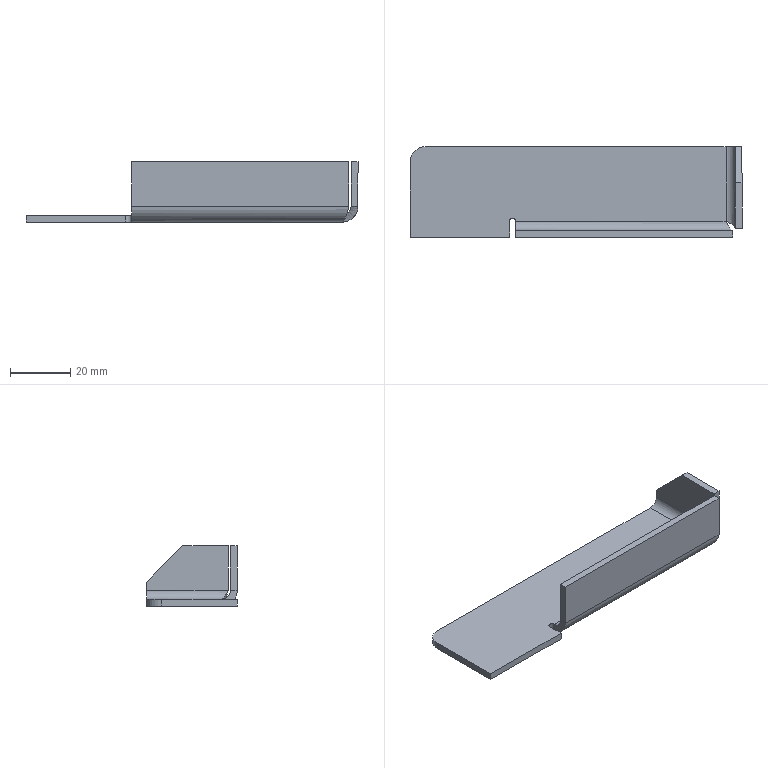Part | SolidWorks | features Chamfer 1, EdgeFlange 1, FlatPattern 1, SMBaseFlange 1, SheetMetal 1 | 1 solid | 27 faces | box 110 x 30 x 20 mm | volume 10965 mm3 | plane 19 | cylinder 6 | spline 2 | commonest cylinder face diameters 6 x2 10.6 x2 2 x1 10 x1
STEP:
#1=CARTESIAN_POINT('',(104.7,30.,-2.3));
#2=VERTEX_POINT('',#1);
#3=CARTESIAN_POINT('',(104.7,5.3,-2.3));
#4=VERTEX_POINT('',#3);
#5=CARTESIAN_POINT('',(104.7,30.,-2.3));
#6=DIRECTION('',(0.,-1.,0.));
#7=VECTOR('',#6,1000.);
#8=LINE('',#5,#7);
#9=EDGE_CURVE('',#2,#4,#8,.T.);
#10=ORIENTED_EDGE('',*,*,#9,.T.);
#11=CARTESIAN_POINT('',(35.,5.3,-2.3));
#12=VERTEX_POINT('',#11);
#13=CARTESIAN_POINT('',(106.993,5.3,-2.3));
#14=DIRECTION('',(-1.,0.,0.));
#15=VECTOR('',#14,1000.);
#16=LINE('',#13,#15);
#17=EDGE_CURVE('',#4,#12,#16,.T.);
#18=ORIENTED_EDGE('',*,*,#17,.T.);
#19=CARTESIAN_POINT('',(33.,5.3,-2.3));
#20=VERTEX_POINT('',#19);
#21=CARTESIAN_POINT('',(34.,5.3,-2.3));
#22=DIRECTION('',(0.,0.,-1.));
#23=DIRECTION('',(1.,0.,0.));
#24=AXIS2_PLACEMENT_3D('',#21,#22,#23);
#25=CIRCLE('',#24,1.);
#26=EDGE_CURVE('',#20,#12,#25,.T.);
#27=ORIENTED_EDGE('',*,*,#26,.F.);
#28=CARTESIAN_POINT('',(33.,0.,-2.3));
#29=VERTEX_POINT('',#28);
#30=CARTESIAN_POINT('',(33.,0.,-2.3));
#31=DIRECTION('',(0.,1.,0.));
#32=VECTOR('',#31,1000.);
#33=LINE('',#30,#32);
#34=EDGE_CURVE('',#29,#20,#33,.T.);
#35=ORIENTED_EDGE('',*,*,#34,.F.);
#36=CARTESIAN_POINT('',(0.,0.,-2.3));
#37=VERTEX_POINT('',#36);
#38=CARTESIAN_POINT('',(0.,0.,-2.3));
#39=DIRECTION('',(1.,0.,0.));
#40=VECTOR('',#39,1000.);
#41=LINE('',#38,#40);
#42=EDGE_CURVE('',#37,#29,#41,.T.);
#43=ORIENTED_EDGE('',*,*,#42,.F.);
#44=CARTESIAN_POINT('',(0.,25.,-2.3));
#45=VERTEX_POINT('',#44);
#46=CARTESIAN_POINT('',(0.,25.,-2.3));
#47=DIRECTION('',(0.,-1.,0.));
#48=VECTOR('',#47,1000.);
#49=LINE('',#46,#48);
#50=EDGE_CURVE('',#45,#37,#49,.T.);
#51=ORIENTED_EDGE('',*,*,#50,.F.);
#52=CARTESIAN_POINT('',(5.,30.,-2.3));
#53=VERTEX_POINT('',#52);
#54=CARTESIAN_POINT('',(5.,25.,-2.3));
#55=DIRECTION('',(0.,0.,1.));
#56=DIRECTION('',(1.,0.,0.));
#57=AXIS2_PLACEMENT_3D('',#54,#55,#56);
#58=CIRCLE('',#57,5.);
#59=EDGE_CURVE('',#53,#45,#58,.T.);
#60=ORIENTED_EDGE('',*,*,#59,.F.);
#61=CARTESIAN_POINT('',(110.,30.,-2.3));
#62=DIRECTION('',(-1.,0.,0.));
#63=VECTOR('',#62,1000.);
#64=LINE('',#61,#63);
#65=EDGE_CURVE('',#2,#53,#64,.T.);
#66=ORIENTED_EDGE('',*,*,#65,.F.);
#67=EDGE_LOOP('',(#10,#18,#27,#35,#43,#51,#60,#66));
#68=FACE_OUTER_BOUND('',#67,.T.);
#69=CARTESIAN_POINT('',(34.,5.3,-2.3));
#70=DIRECTION('',(0.,0.,1.));
#71=DIRECTION('',(1.,0.,0.));
#72=AXIS2_PLACEMENT_3D('',#69,#70,#71);
#73=PLANE('',#72);
#74=ADVANCED_FACE('',(#68),#73,.F.);
#75=CARTESIAN_POINT('',(104.7,5.3,0.));
#76=VERTEX_POINT('',#75);
#77=CARTESIAN_POINT('',(35.,5.3,0.));
#78=VERTEX_POINT('',#77);
#79=CARTESIAN_POINT('',(106.993,5.3,0.));
#80=DIRECTION('',(-1.,0.,0.));
#81=VECTOR('',#80,1000.);
#82=LINE('',#79,#81);
#83=EDGE_CURVE('',#76,#78,#82,.T.);
#84=ORIENTED_EDGE('',*,*,#83,.F.);
#85=CARTESIAN_POINT('',(104.7,30.,0.));
#86=VERTEX_POINT('',#85);
#87=CARTESIAN_POINT('',(104.7,30.,0.));
#88=DIRECTION('',(0.,-1.,0.));
#89=VECTOR('',#88,1000.);
#90=LINE('',#87,#89);
#91=EDGE_CURVE('',#86,#76,#90,.T.);
#92=ORIENTED_EDGE('',*,*,#91,.F.);
#93=CARTESIAN_POINT('',(5.,30.,0.));
#94=VERTEX_POINT('',#93);
#95=CARTESIAN_POINT('',(110.,30.,0.));
#96=DIRECTION('',(-1.,0.,0.));
#97=VECTOR('',#96,1000.);
#98=LINE('',#95,#97);
#99=EDGE_CURVE('',#86,#94,#98,.T.);
#100=ORIENTED_EDGE('',*,*,#99,.T.);
#101=CARTESIAN_POINT('',(0.,25.,0.));
#102=VERTEX_POINT('',#101);
#103=CARTESIAN_POINT('',(5.,25.,0.));
#104=DIRECTION('',(0.,0.,1.));
#105=DIRECTION('',(1.,0.,0.));
#106=AXIS2_PLACEMENT_3D('',#103,#104,#105);
#107=CIRCLE('',#106,5.);
#108=EDGE_CURVE('',#94,#102,#107,.T.);
#109=ORIENTED_EDGE('',*,*,#108,.T.);
#110=CARTESIAN_POINT('',(0.,0.,0.));
#111=VERTEX_POINT('',#110);
#112=CARTESIAN_POINT('',(0.,25.,0.));
#113=DIRECTION('',(0.,-1.,0.));
#114=VECTOR('',#113,1000.);
#115=LINE('',#112,#114);
#116=EDGE_CURVE('',#102,#111,#115,.T.);
#117=ORIENTED_EDGE('',*,*,#116,.T.);
#118=CARTESIAN_POINT('',(33.,0.,0.));
#119=VERTEX_POINT('',#118);
#120=CARTESIAN_POINT('',(0.,0.,0.));
#121=DIRECTION('',(1.,0.,0.));
#122=VECTOR('',#121,1000.);
#123=LINE('',#120,#122);
#124=EDGE_CURVE('',#111,#119,#123,.T.);
#125=ORIENTED_EDGE('',*,*,#124,.T.);
#126=CARTESIAN_POINT('',(33.,5.3,0.));
#127=VERTEX_POINT('',#126);
#128=CARTESIAN_POINT('',(33.,0.,0.));
#129=DIRECTION('',(0.,1.,0.));
#130=VECTOR('',#129,1000.);
#131=LINE('',#128,#130);
#132=EDGE_CURVE('',#119,#127,#131,.T.);
#133=ORIENTED_EDGE('',*,*,#132,.T.);
#134=CARTESIAN_POINT('',(34.,5.3,0.));
#135=DIRECTION('',(0.,0.,-1.));
#136=DIRECTION('',(1.,0.,0.));
#137=AXIS2_PLACEMENT_3D('',#134,#135,#136);
#138=CIRCLE('',#137,1.);
#139=EDGE_CURVE('',#127,#78,#138,.T.);
#140=ORIENTED_EDGE('',*,*,#139,.T.);
#141=EDGE_LOOP('',(#84,#92,#100,#109,#117,#125,#133,#140));
#142=FACE_OUTER_BOUND('',#141,.T.);
#143=CARTESIAN_POINT('',(34.,5.3,0.));
#144=DIRECTION('',(0.,0.,1.));
#145=DIRECTION('',(1.,0.,0.));
#146=AXIS2_PLACEMENT_3D('',#143,#144,#145);
#147=PLANE('',#146);
#148=ADVANCED_FACE('',(#142),#147,.T.);
#149=ORIENTED_EDGE('',*,*,#99,.F.);
#150=CARTESIAN_POINT('',(104.7,30.,0.));
#151=DIRECTION('',(0.,0.,-1.));
#152=VECTOR('',#151,1000.);
#153=LINE('',#150,#152);
#154=EDGE_CURVE('',#86,#2,#153,.T.);
#155=ORIENTED_EDGE('',*,*,#154,.T.);
#156=ORIENTED_EDGE('',*,*,#65,.T.);
#157=CARTESIAN_POINT('',(5.,30.,-2.3));
#158=DIRECTION('',(0.,0.,1.));
#159=VECTOR('',#158,1000.);
#160=LINE('',#157,#159);
#161=EDGE_CURVE('',#53,#94,#160,.T.);
#162=ORIENTED_EDGE('',*,*,#161,.T.);
#163=EDGE_LOOP('',(#149,#155,#156,#162));
#164=FACE_OUTER_BOUND('',#163,.T.);
#165=CARTESIAN_POINT('',(110.,30.,-2.3));
#166=DIRECTION('',(0.,1.,0.));
#167=DIRECTION('',(-1.,0.,0.));
#168=AXIS2_PLACEMENT_3D('',#165,#166,#167);
#169=PLANE('',#168);
#170=ADVANCED_FACE('',(#164),#169,.T.);
#171=ORIENTED_EDGE('',*,*,#116,.F.);
#172=CARTESIAN_POINT('',(0.,25.,-2.3));
#173=DIRECTION('',(0.,0.,1.));
#174=VECTOR('',#173,1000.);
#175=LINE('',#172,#174);
#176=EDGE_CURVE('',#45,#102,#175,.T.);
#177=ORIENTED_EDGE('',*,*,#176,.F.);
#178=ORIENTED_EDGE('',*,*,#50,.T.);
#179=CARTESIAN_POINT('',(0.,0.,-2.3));
#180=DIRECTION('',(0.,0.,1.));
#181=VECTOR('',#180,1000.);
#182=LINE('',#179,#181);
#183=EDGE_CURVE('',#37,#111,#182,.T.);
#184=ORIENTED_EDGE('',*,*,#183,.T.);
#185=EDGE_LOOP('',(#171,#177,#178,#184));
#186=FACE_OUTER_BOUND('',#185,.T.);
#187=CARTESIAN_POINT('',(0.,25.,-2.3));
#188=DIRECTION('',(-1.,0.,0.));
#189=DIRECTION('',(0.,0.,1.));
#190=AXIS2_PLACEMENT_3D('',#187,#188,#189);
#191=PLANE('',#190);
#192=ADVANCED_FACE('',(#186),#191,.T.);
#193=ORIENTED_EDGE('',*,*,#108,.F.);
#194=ORIENTED_EDGE('',*,*,#161,.F.);
#195=ORIENTED_EDGE('',*,*,#59,.T.);
#196=ORIENTED_EDGE('',*,*,#176,.T.);
#197=EDGE_LOOP('',(#193,#194,#195,#196));
#198=FACE_OUTER_BOUND('',#197,.T.);
#199=CARTESIAN_POINT('',(5.,25.,-2.3));
#200=DIRECTION('',(0.,0.,1.));
#201=DIRECTION('',(1.,0.,0.));
#202=AXIS2_PLACEMENT_3D('',#199,#200,#201);
#203=CYLINDRICAL_SURFACE('',#202,5.);
#204=ADVANCED_FACE('',(#198),#203,.T.);
#205=ORIENTED_EDGE('',*,*,#139,.F.);
#206=CARTESIAN_POINT('',(33.,5.3,-2.3));
#207=DIRECTION('',(0.,0.,1.));
#208=VECTOR('',#207,1000.);
#209=LINE('',#206,#208);
#210=EDGE_CURVE('',#20,#127,#209,.T.);
#211=ORIENTED_EDGE('',*,*,#210,.F.);
#212=ORIENTED_EDGE('',*,*,#26,.T.);
#213=CARTESIAN_POINT('',(35.,5.3,-2.3));
#214=DIRECTION('',(0.,0.,1.));
#215=VECTOR('',#214,1000.);
#216=LINE('',#213,#215);
#217=EDGE_CURVE('',#12,#78,#216,.T.);
#218=ORIENTED_EDGE('',*,*,#217,.T.);
#219=EDGE_LOOP('',(#205,#211,#212,#218));
#220=FACE_OUTER_BOUND('',#219,.T.);
#221=CARTESIAN_POINT('',(34.,5.3,-2.3));
#222=DIRECTION('',(0.,0.,1.));
#223=DIRECTION('',(1.,0.,0.));
#224=AXIS2_PLACEMENT_3D('',#221,#222,#223);
#225=CYLINDRICAL_SURFACE('',#224,1.);
#226=ADVANCED_FACE('',(#220),#225,.F.);
#227=ORIENTED_EDGE('',*,*,#132,.F.);
#228=CARTESIAN_POINT('',(33.,0.,-2.3));
#229=DIRECTION('',(0.,0.,1.));
#230=VECTOR('',#229,1000.);
#231=LINE('',#228,#230);
#232=EDGE_CURVE('',#29,#119,#231,.T.);
#233=ORIENTED_EDGE('',*,*,#232,.F.);
#234=ORIENTED_EDGE('',*,*,#34,.T.);
#235=ORIENTED_EDGE('',*,*,#210,.T.);
#236=EDGE_LOOP('',(#227,#233,#234,#235));
#237=FACE_OUTER_BOUND('',#236,.T.);
#238=CARTESIAN_POINT('',(33.,0.,-2.3));
#239=DIRECTION('',(1.,0.,0.));
#240=DIRECTION('',(0.,1.,0.));
#241=AXIS2_PLACEMENT_3D('',#238,#239,#240);
#242=PLANE('',#241);
#243=ADVANCED_FACE('',(#237),#242,.T.);
#244=ORIENTED_EDGE('',*,*,#124,.F.);
#245=ORIENTED_EDGE('',*,*,#183,.F.);
#246=ORIENTED_EDGE('',*,*,#42,.T.);
#247=ORIENTED_EDGE('',*,*,#232,.T.);
#248=EDGE_LOOP('',(#244,#245,#246,#247));
#249=FACE_OUTER_BOUND('',#248,.T.);
#250=CARTESIAN_POINT('',(0.,0.,-2.3));
#251=DIRECTION('',(0.,-1.,0.));
#252=DIRECTION('',(0.,0.,-1.));
#253=AXIS2_PLACEMENT_3D('',#250,#251,#252);
#254=PLANE('',#253);
#255=ADVANCED_FACE('',(#249),#254,.T.);
#256=CARTESIAN_POINT('',(35.,2.3,3.));
#257=VERTEX_POINT('',#256);
#258=CARTESIAN_POINT('',(35.,0.,3.));
#259=VERTEX_POINT('',#258);
#260=CARTESIAN_POINT('',(35.,0.,3.));
#261=DIRECTION('',(0.,-1.,0.));
#262=VECTOR('',#261,1000.);
#263=LINE('',#260,#262);
#264=EDGE_CURVE('',#257,#259,#263,.T.);
#265=ORIENTED_EDGE('',*,*,#264,.F.);
#266=CARTESIAN_POINT('',(35.,5.3,3.));
#267=DIRECTION('',(-1.,0.,0.));
#268=DIRECTION('',(0.,0.,-1.));
#269=AXIS2_PLACEMENT_3D('',#266,#267,#268);
#270=CIRCLE('',#269,3.);
#271=EDGE_CURVE('',#78,#257,#270,.T.);
#272=ORIENTED_EDGE('',*,*,#271,.F.);
#273=ORIENTED_EDGE('',*,*,#217,.F.);
#274=CARTESIAN_POINT('',(35.,5.3,3.));
#275=DIRECTION('',(-1.,0.,0.));
#276=DIRECTION('',(0.,0.,-1.));
#277=AXIS2_PLACEMENT_3D('',#274,#275,#276);
#278=CIRCLE('',#277,5.3);
#279=EDGE_CURVE('',#12,#259,#278,.T.);
#280=ORIENTED_EDGE('',*,*,#279,.T.);
#281=EDGE_LOOP('',(#265,#272,#273,#280));
#282=FACE_OUTER_BOUND('',#281,.T.);
#283=CARTESIAN_POINT('',(35.,5.3,3.));
#284=DIRECTION('',(-1.,0.,0.));
#285=DIRECTION('',(0.,0.,1.));
#286=AXIS2_PLACEMENT_3D('',#283,#284,#285);
#287=PLANE('',#286);
#288=ADVANCED_FACE('',(#282),#287,.T.);
#289=CARTESIAN_POINT('',(106.993,2.3,3.));
#290=VERTEX_POINT('',#289);
#291=CARTESIAN_POINT('',(106.993,2.3,3.));
#292=CARTESIAN_POINT('',(106.897,2.3,2.802));
#293=CARTESIAN_POINT('',(106.801,2.319,2.607));
#294=CARTESIAN_POINT('',(106.611,2.396,2.223));
#295=CARTESIAN_POINT('',(106.515,2.453,2.033));
#296=CARTESIAN_POINT('',(106.323,2.604,1.669));
#297=CARTESIAN_POINT('',(106.229,2.697,1.497));
#298=CARTESIAN_POINT('',(106.038,2.914,1.171));
#299=CARTESIAN_POINT('',(105.942,3.04,1.018));
#300=CARTESIAN_POINT('',(105.751,3.318,0.7394));
#301=CARTESIAN_POINT('',(105.656,3.469,0.6154));
#302=CARTESIAN_POINT('',(105.466,3.794,0.3979));
#303=CARTESIAN_POINT('',(105.369,3.97,0.3037));
#304=CARTESIAN_POINT('',(105.178,4.333,0.1534));
#305=CARTESIAN_POINT('',(105.083,4.52,0.09658));
#306=CARTESIAN_POINT('',(104.893,4.904,0.01983));
#307=CARTESIAN_POINT('',(104.796,5.102,0.));
#308=CARTESIAN_POINT('',(104.7,5.3,0.));
#309=B_SPLINE_CURVE_WITH_KNOTS('',3,(#291,#292,#293,#294,#295,#296,#297,#298,#299,#300,#301,#302,#303,#304,#305,#306,#307,#308),.UNSPECIFIED.,.F.,.F.,(4,2,2,2,2,2,2,2,4),(0.,0.0006524,0.001305,0.001957,0.00261,0.003262,0.003914,0.004567,0.005219),.UNSPECIFIED.);
#310=EDGE_CURVE('',#290,#76,#309,.T.);
#311=ORIENTED_EDGE('',*,*,#310,.F.);
#312=CARTESIAN_POINT('',(106.993,0.,3.));
#313=VERTEX_POINT('',#312);
#314=CARTESIAN_POINT('',(106.993,2.3,3.));
#315=DIRECTION('',(0.,1.,0.));
#316=VECTOR('',#315,1000.);
#317=LINE('',#314,#316);
#318=EDGE_CURVE('',#313,#290,#317,.T.);
#319=ORIENTED_EDGE('',*,*,#318,.F.);
#320=CARTESIAN_POINT('',(106.993,0.,3.));
#321=CARTESIAN_POINT('',(106.897,0.,2.65));
#322=CARTESIAN_POINT('',(106.802,0.03435,2.306));
#323=CARTESIAN_POINT('',(106.659,0.1352,1.798));
#324=CARTESIAN_POINT('',(106.612,0.1771,1.63));
#325=CARTESIAN_POINT('',(106.516,0.2777,1.298));
#326=CARTESIAN_POINT('',(106.468,0.3368,1.133));
#327=CARTESIAN_POINT('',(106.324,0.5364,0.6506));
#328=CARTESIAN_POINT('',(106.229,0.6993,0.3462));
#329=CARTESIAN_POINT('',(106.039,1.083,-0.2288));
#330=CARTESIAN_POINT('',(105.942,1.306,-0.5016));
#331=CARTESIAN_POINT('',(105.752,1.796,-0.9914));
#332=CARTESIAN_POINT('',(105.657,2.063,-1.211));
#333=CARTESIAN_POINT('',(105.466,2.639,-1.597));
#334=CARTESIAN_POINT('',(105.369,2.949,-1.763));
#335=CARTESIAN_POINT('',(105.179,3.587,-2.027));
#336=CARTESIAN_POINT('',(105.084,3.918,-2.128));
#337=CARTESIAN_POINT('',(104.893,4.601,-2.265));
#338=CARTESIAN_POINT('',(104.796,4.95,-2.3));
#339=CARTESIAN_POINT('',(104.7,5.3,-2.3));
#340=B_SPLINE_CURVE_WITH_KNOTS('',3,(#320,#321,#322,#323,#324,#325,#326,#327,#328,#329,#330,#331,#332,#333,#334,#335,#336,#337,#338,#339),.UNSPECIFIED.,.F.,.F.,(4,2,2,2,2,2,2,2,2,4),(0.,0.001073,0.00161,0.002147,0.00322,0.004294,0.005367,0.006441,0.007514,0.008588),.UNSPECIFIED.);
#341=EDGE_CURVE('',#313,#4,#340,.T.);
#342=ORIENTED_EDGE('',*,*,#341,.T.);
#343=CARTESIAN_POINT('',(104.7,5.3,0.));
#344=DIRECTION('',(0.,0.,-1.));
#345=VECTOR('',#344,1000.);
#346=LINE('',#343,#345);
#347=EDGE_CURVE('',#76,#4,#346,.T.);
#348=ORIENTED_EDGE('',*,*,#347,.F.);
#349=EDGE_LOOP('',(#311,#319,#342,#348));
#350=FACE_OUTER_BOUND('',#349,.T.);
#351=CARTESIAN_POINT('',(106.993,-0.023,3.));
#352=CARTESIAN_POINT('',(106.802,-0.023,2.303));
#353=CARTESIAN_POINT('',(106.611,0.1155,1.607));
#354=CARTESIAN_POINT('',(106.229,0.6488,0.3192));
#355=CARTESIAN_POINT('',(106.038,1.043,-0.2712));
#356=CARTESIAN_POINT('',(105.655,2.029,-1.257));
#357=CARTESIAN_POINT('',(105.464,2.619,-1.651));
#358=CARTESIAN_POINT('',(105.082,3.907,-2.184));
#359=CARTESIAN_POINT('',(104.891,4.603,-2.323));
#360=CARTESIAN_POINT('',(104.7,5.3,-2.323));
#361=CARTESIAN_POINT('',(106.993,0.,3.));
#362=CARTESIAN_POINT('',(106.802,0.,2.306));
#363=CARTESIAN_POINT('',(106.611,0.1379,1.613));
#364=CARTESIAN_POINT('',(106.229,0.6689,0.3308));
#365=CARTESIAN_POINT('',(106.038,1.062,-0.2571));
#366=CARTESIAN_POINT('',(105.655,2.043,-1.238));
#367=CARTESIAN_POINT('',(105.464,2.631,-1.631));
#368=CARTESIAN_POINT('',(105.082,3.913,-2.162));
#369=CARTESIAN_POINT('',(104.891,4.606,-2.3));
#370=CARTESIAN_POINT('',(104.7,5.3,-2.3));
#371=CARTESIAN_POINT('',(106.993,2.3,3.));
#372=CARTESIAN_POINT('',(106.802,2.3,2.607));
#373=CARTESIAN_POINT('',(106.611,2.378,2.215));
#374=CARTESIAN_POINT('',(106.229,2.679,1.489));
#375=CARTESIAN_POINT('',(106.038,2.901,1.156));
#376=CARTESIAN_POINT('',(105.655,3.456,0.601));
#377=CARTESIAN_POINT('',(105.464,3.789,0.3786));
#378=CARTESIAN_POINT('',(105.082,4.515,0.07808));
#379=CARTESIAN_POINT('',(104.891,4.907,0.));
#380=CARTESIAN_POINT('',(104.7,5.3,0.));
#381=CARTESIAN_POINT('',(106.993,2.323,3.));
#382=CARTESIAN_POINT('',(106.802,2.323,2.61));
#383=CARTESIAN_POINT('',(106.611,2.401,2.221));
#384=CARTESIAN_POINT('',(106.229,2.699,1.501));
#385=CARTESIAN_POINT('',(106.038,2.92,1.171));
#386=CARTESIAN_POINT('',(105.655,3.471,0.6196));
#387=CARTESIAN_POINT('',(105.464,3.801,0.3989));
#388=CARTESIAN_POINT('',(105.082,4.521,0.1007));
#389=CARTESIAN_POINT('',(104.891,4.91,0.02323));
#390=CARTESIAN_POINT('',(104.7,5.3,0.02323));
#391=B_SPLINE_SURFACE_WITH_KNOTS('',1,3,((#351,#352,#353,#354,#355,#356,#357,#358,#359,#360),(#361,#362,#363,#364,#365,#366,#367,#368,#369,#370),(#371,#372,#373,#374,#375,#376,#377,#378,#379,#380),(#381,#382,#383,#384,#385,#386,#387,#388,#389,#390)),.UNSPECIFIED.,.F.,.F.,.F.,(2,1,1,2),(4,2,2,2,4),(-0.01,0.,1.,1.01),(0.,0.25,0.5,0.75,1.),.UNSPECIFIED.);
#392=ADVANCED_FACE('',(#350),#391,.F.);
#393=ORIENTED_EDGE('',*,*,#17,.F.);
#394=ORIENTED_EDGE('',*,*,#341,.F.);
#395=CARTESIAN_POINT('',(35.,0.,3.));
#396=DIRECTION('',(-1.,0.,0.));
#397=VECTOR('',#396,1000.);
#398=LINE('',#395,#397);
#399=EDGE_CURVE('',#313,#259,#398,.T.);
#400=ORIENTED_EDGE('',*,*,#399,.T.);
#401=ORIENTED_EDGE('',*,*,#279,.F.);
#402=EDGE_LOOP('',(#393,#394,#400,#401));
#403=FACE_OUTER_BOUND('',#402,.T.);
#404=CARTESIAN_POINT('',(106.993,5.3,3.));
#405=DIRECTION('',(1.,0.,0.));
#406=DIRECTION('',(0.,-1.,0.));
#407=AXIS2_PLACEMENT_3D('',#404,#405,#406);
#408=CYLINDRICAL_SURFACE('',#407,5.3);
#409=ADVANCED_FACE('',(#403),#408,.T.);
#410=ORIENTED_EDGE('',*,*,#83,.T.);
#411=ORIENTED_EDGE('',*,*,#271,.T.);
#412=CARTESIAN_POINT('',(35.,2.3,3.));
#413=DIRECTION('',(1.,0.,0.));
#414=VECTOR('',#413,1000.);
#415=LINE('',#412,#414);
#416=EDGE_CURVE('',#257,#290,#415,.T.);
#417=ORIENTED_EDGE('',*,*,#416,.T.);
#418=ORIENTED_EDGE('',*,*,#310,.T.);
#419=EDGE_LOOP('',(#410,#411,#417,#418));
#420=FACE_OUTER_BOUND('',#419,.T.);
#421=CARTESIAN_POINT('',(106.993,5.3,3.));
#422=DIRECTION('',(1.,0.,0.));
#423=DIRECTION('',(0.,-1.,0.));
#424=AXIS2_PLACEMENT_3D('',#421,#422,#423);
#425=CYLINDRICAL_SURFACE('',#424,3.);
#426=ADVANCED_FACE('',(#420),#425,.F.);
#427=ORIENTED_EDGE('',*,*,#264,.T.);
#428=CARTESIAN_POINT('',(35.,0.,17.7));
#429=VERTEX_POINT('',#428);
#430=CARTESIAN_POINT('',(35.,0.,0.));
#431=DIRECTION('',(0.,0.,-1.));
#432=VECTOR('',#431,1000.);
#433=LINE('',#430,#432);
#434=EDGE_CURVE('',#429,#259,#433,.T.);
#435=ORIENTED_EDGE('',*,*,#434,.F.);
#436=CARTESIAN_POINT('',(35.,2.3,17.7));
#437=VERTEX_POINT('',#436);
#438=CARTESIAN_POINT('',(35.,0.,17.7));
#439=DIRECTION('',(0.,1.,0.));
#440=VECTOR('',#439,1000.);
#441=LINE('',#438,#440);
#442=EDGE_CURVE('',#429,#437,#441,.T.);
#443=ORIENTED_EDGE('',*,*,#442,.T.);
#444=CARTESIAN_POINT('',(35.,2.3,0.));
#445=DIRECTION('',(0.,0.,-1.));
#446=VECTOR('',#445,1000.);
#447=LINE('',#444,#446);
#448=EDGE_CURVE('',#437,#257,#447,.T.);
#449=ORIENTED_EDGE('',*,*,#448,.T.);
#450=EDGE_LOOP('',(#427,#435,#443,#449));
#451=FACE_OUTER_BOUND('',#450,.T.);
#452=CARTESIAN_POINT('',(35.,0.,0.));
#453=DIRECTION('',(1.,0.,0.));
#454=DIRECTION('',(0.,0.,-1.));
#455=AXIS2_PLACEMENT_3D('',#452,#453,#454);
#456=PLANE('',#455);
#457=ADVANCED_FACE('',(#451),#456,.F.);
#458=ORIENTED_EDGE('',*,*,#399,.F.);
#459=CARTESIAN_POINT('',(106.993,0.,17.7));
#460=VERTEX_POINT('',#459);
#461=CARTESIAN_POINT('',(106.993,0.,0.));
#462=DIRECTION('',(0.,0.,1.));
#463=VECTOR('',#462,1000.);
#464=LINE('',#461,#463);
#465=EDGE_CURVE('',#313,#460,#464,.T.);
#466=ORIENTED_EDGE('',*,*,#465,.T.);
#467=CARTESIAN_POINT('',(0.,0.,17.7));
#468=DIRECTION('',(-1.,0.,0.));
#469=VECTOR('',#468,1000.);
#470=LINE('',#467,#469);
#471=EDGE_CURVE('',#460,#429,#470,.T.);
#472=ORIENTED_EDGE('',*,*,#471,.T.);
#473=ORIENTED_EDGE('',*,*,#434,.T.);
#474=EDGE_LOOP('',(#458,#466,#472,#473));
#475=FACE_OUTER_BOUND('',#474,.T.);
#476=CARTESIAN_POINT('',(0.,0.,0.));
#477=DIRECTION('',(0.,1.,0.));
#478=DIRECTION('',(0.,0.,1.));
#479=AXIS2_PLACEMENT_3D('',#476,#477,#478);
#480=PLANE('',#479);
#481=ADVANCED_FACE('',(#475),#480,.F.);
#482=CARTESIAN_POINT('',(106.993,2.3,17.7));
#483=VERTEX_POINT('',#482);
#484=CARTESIAN_POINT('',(106.993,2.3,0.));
#485=DIRECTION('',(0.,0.,1.));
#486=VECTOR('',#485,1000.);
#487=LINE('',#484,#486);
#488=EDGE_CURVE('',#290,#483,#487,.T.);
#489=ORIENTED_EDGE('',*,*,#488,.F.);
#490=ORIENTED_EDGE('',*,*,#416,.F.);
#491=ORIENTED_EDGE('',*,*,#448,.F.);
#492=CARTESIAN_POINT('',(35.,2.3,17.7));
#493=DIRECTION('',(-1.,0.,0.));
#494=VECTOR('',#493,1000.);
#495=LINE('',#492,#494);
#496=EDGE_CURVE('',#483,#437,#495,.T.);
#497=ORIENTED_EDGE('',*,*,#496,.F.);
#498=EDGE_LOOP('',(#489,#490,#491,#497));
#499=FACE_OUTER_BOUND('',#498,.T.);
#500=CARTESIAN_POINT('',(0.,2.3,0.));
#501=DIRECTION('',(0.,1.,0.));
#502=DIRECTION('',(0.,0.,1.));
#503=AXIS2_PLACEMENT_3D('',#500,#501,#502);
#504=PLANE('',#503);
#505=ADVANCED_FACE('',(#499),#504,.T.);
#506=ORIENTED_EDGE('',*,*,#471,.F.);
#507=CARTESIAN_POINT('',(106.993,0.,17.7));
#508=DIRECTION('',(0.,1.,0.));
#509=VECTOR('',#508,1000.);
#510=LINE('',#507,#509);
#511=EDGE_CURVE('',#460,#483,#510,.T.);
#512=ORIENTED_EDGE('',*,*,#511,.T.);
#513=ORIENTED_EDGE('',*,*,#496,.T.);
#514=ORIENTED_EDGE('',*,*,#442,.F.);
#515=EDGE_LOOP('',(#506,#512,#513,#514));
#516=FACE_OUTER_BOUND('',#515,.T.);
#517=CARTESIAN_POINT('',(35.,0.,17.7));
#518=DIRECTION('',(0.,0.,-1.));
#519=DIRECTION('',(0.,1.,0.));
#520=AXIS2_PLACEMENT_3D('',#517,#518,#519);
#521=PLANE('',#520);
#522=ADVANCED_FACE('',(#516),#521,.F.);
#523=ORIENTED_EDGE('',*,*,#511,.F.);
#524=ORIENTED_EDGE('',*,*,#465,.F.);
#525=ORIENTED_EDGE('',*,*,#318,.T.);
#526=ORIENTED_EDGE('',*,*,#488,.T.);
#527=EDGE_LOOP('',(#523,#524,#525,#526));
#528=FACE_OUTER_BOUND('',#527,.T.);
#529=CARTESIAN_POINT('',(106.993,2.3,0.));
#530=DIRECTION('',(-1.,0.,0.));
#531=DIRECTION('',(0.,0.,1.));
#532=AXIS2_PLACEMENT_3D('',#529,#530,#531);
#533=PLANE('',#532);
#534=ADVANCED_FACE('',(#528),#533,.F.);
#535=CARTESIAN_POINT('',(110.,3.007,3.));
#536=VERTEX_POINT('',#535);
#537=CARTESIAN_POINT('',(107.7,3.007,3.));
#538=VERTEX_POINT('',#537);
#539=CARTESIAN_POINT('',(107.7,3.007,3.));
#540=DIRECTION('',(-1.,0.,0.));
#541=VECTOR('',#540,1000.);
#542=LINE('',#539,#541);
#543=EDGE_CURVE('',#536,#538,#542,.T.);
#544=ORIENTED_EDGE('',*,*,#543,.T.);
#545=CARTESIAN_POINT('',(104.7,5.3,0.));
#546=CARTESIAN_POINT('',(104.898,5.204,0.));
#547=CARTESIAN_POINT('',(105.093,5.109,0.01948));
#548=CARTESIAN_POINT('',(105.477,4.918,0.09577));
#549=CARTESIAN_POINT('',(105.667,4.822,0.1532));
#550=CARTESIAN_POINT('',(106.031,4.63,0.3042));
#551=CARTESIAN_POINT('',(106.203,4.536,0.3966));
#552=CARTESIAN_POINT('',(106.529,4.345,0.6136));
#553=CARTESIAN_POINT('',(106.682,4.249,0.7397));
#554=CARTESIAN_POINT('',(106.961,4.058,1.018));
#555=CARTESIAN_POINT('',(107.085,3.963,1.169));
#556=CARTESIAN_POINT('',(107.302,3.773,1.494));
#557=CARTESIAN_POINT('',(107.396,3.676,1.67));
#558=CARTESIAN_POINT('',(107.547,3.485,2.033));
#559=CARTESIAN_POINT('',(107.603,3.39,2.22));
#560=CARTESIAN_POINT('',(107.68,3.2,2.604));
#561=CARTESIAN_POINT('',(107.7,3.103,2.802));
#562=CARTESIAN_POINT('',(107.7,3.007,3.));
#563=B_SPLINE_CURVE_WITH_KNOTS('',3,(#545,#546,#547,#548,#549,#550,#551,#552,#553,#554,#555,#556,#557,#558,#559,#560,#561,#562),.UNSPECIFIED.,.F.,.F.,(4,2,2,2,2,2,2,2,4),(0.,0.0006524,0.001305,0.001957,0.00261,0.003262,0.003914,0.004567,0.005219),.UNSPECIFIED.);
#564=EDGE_CURVE('',#76,#538,#563,.T.);
#565=ORIENTED_EDGE('',*,*,#564,.F.);
#566=ORIENTED_EDGE('',*,*,#347,.T.);
#567=CARTESIAN_POINT('',(104.7,5.3,-2.3));
#568=CARTESIAN_POINT('',(105.05,5.204,-2.3));
#569=CARTESIAN_POINT('',(105.394,5.109,-2.266));
#570=CARTESIAN_POINT('',(105.902,4.966,-2.165));
#571=CARTESIAN_POINT('',(106.07,4.919,-2.123));
#572=CARTESIAN_POINT('',(106.402,4.823,-2.022));
#573=CARTESIAN_POINT('',(106.567,4.775,-1.963));
#574=CARTESIAN_POINT('',(107.049,4.631,-1.764));
#575=CARTESIAN_POINT('',(107.354,4.536,-1.601));
#576=CARTESIAN_POINT('',(107.929,4.346,-1.217));
#577=CARTESIAN_POINT('',(108.202,4.249,-0.9936));
#578=CARTESIAN_POINT('',(108.691,4.059,-0.504));
#579=CARTESIAN_POINT('',(108.911,3.964,-0.2375));
#580=CARTESIAN_POINT('',(109.297,3.773,0.3388));
#581=CARTESIAN_POINT('',(109.463,3.676,0.6493));
#582=CARTESIAN_POINT('',(109.727,3.486,1.287));
#583=CARTESIAN_POINT('',(109.828,3.392,1.618));
#584=CARTESIAN_POINT('',(109.965,3.2,2.301));
#585=CARTESIAN_POINT('',(110.,3.103,2.65));
#586=CARTESIAN_POINT('',(110.,3.007,3.));
#587=B_SPLINE_CURVE_WITH_KNOTS('',3,(#567,#568,#569,#570,#571,#572,#573,#574,#575,#576,#577,#578,#579,#580,#581,#582,#583,#584,#585,#586),.UNSPECIFIED.,.F.,.F.,(4,2,2,2,2,2,2,2,2,4),(0.,0.001073,0.00161,0.002147,0.00322,0.004294,0.005367,0.006441,0.007514,0.008588),.UNSPECIFIED.);
#588=EDGE_CURVE('',#4,#536,#587,.T.);
#589=ORIENTED_EDGE('',*,*,#588,.T.);
#590=EDGE_LOOP('',(#544,#565,#566,#589));
#591=FACE_OUTER_BOUND('',#590,.T.);
#592=CARTESIAN_POINT('',(104.7,5.3,-2.323));
#593=CARTESIAN_POINT('',(105.397,5.109,-2.323));
#594=CARTESIAN_POINT('',(106.093,4.918,-2.184));
#595=CARTESIAN_POINT('',(107.381,4.536,-1.651));
#596=CARTESIAN_POINT('',(107.971,4.345,-1.257));
#597=CARTESIAN_POINT('',(108.957,3.962,-0.2712));
#598=CARTESIAN_POINT('',(109.351,3.771,0.3192));
#599=CARTESIAN_POINT('',(109.884,3.389,1.607));
#600=CARTESIAN_POINT('',(110.023,3.198,2.303));
#601=CARTESIAN_POINT('',(110.023,3.007,3.));
#602=CARTESIAN_POINT('',(104.7,5.3,-2.3));
#603=CARTESIAN_POINT('',(105.394,5.109,-2.3));
#604=CARTESIAN_POINT('',(106.087,4.918,-2.162));
#605=CARTESIAN_POINT('',(107.369,4.536,-1.631));
#606=CARTESIAN_POINT('',(107.957,4.345,-1.238));
#607=CARTESIAN_POINT('',(108.938,3.962,-0.2571));
#608=CARTESIAN_POINT('',(109.331,3.771,0.3308));
#609=CARTESIAN_POINT('',(109.862,3.389,1.613));
#610=CARTESIAN_POINT('',(110.,3.198,2.306));
#611=CARTESIAN_POINT('',(110.,3.007,3.));
#612=CARTESIAN_POINT('',(104.7,5.3,0.));
#613=CARTESIAN_POINT('',(105.093,5.109,0.));
#614=CARTESIAN_POINT('',(105.485,4.918,0.07808));
#615=CARTESIAN_POINT('',(106.211,4.536,0.3786));
#616=CARTESIAN_POINT('',(106.544,4.345,0.601));
#617=CARTESIAN_POINT('',(107.099,3.962,1.156));
#618=CARTESIAN_POINT('',(107.321,3.771,1.489));
#619=CARTESIAN_POINT('',(107.622,3.389,2.215));
#620=CARTESIAN_POINT('',(107.7,3.198,2.607));
#621=CARTESIAN_POINT('',(107.7,3.007,3.));
#622=CARTESIAN_POINT('',(104.7,5.3,0.02323));
#623=CARTESIAN_POINT('',(105.09,5.109,0.02323));
#624=CARTESIAN_POINT('',(105.479,4.918,0.1007));
#625=CARTESIAN_POINT('',(106.199,4.536,0.3989));
#626=CARTESIAN_POINT('',(106.529,4.345,0.6196));
#627=CARTESIAN_POINT('',(107.08,3.962,1.171));
#628=CARTESIAN_POINT('',(107.301,3.771,1.501));
#629=CARTESIAN_POINT('',(107.599,3.389,2.221));
#630=CARTESIAN_POINT('',(107.677,3.198,2.61));
#631=CARTESIAN_POINT('',(107.677,3.007,3.));
#632=B_SPLINE_SURFACE_WITH_KNOTS('',1,3,((#592,#593,#594,#595,#596,#597,#598,#599,#600,#601),(#602,#603,#604,#605,#606,#607,#608,#609,#610,#611),(#612,#613,#614,#615,#616,#617,#618,#619,#620,#621),(#622,#623,#624,#625,#626,#627,#628,#629,#630,#631)),.UNSPECIFIED.,.F.,.F.,.F.,(2,1,1,2),(4,2,2,2,4),(-0.01,0.,1.,1.01),(0.,0.25,0.5,0.75,1.),.UNSPECIFIED.);
#633=ADVANCED_FACE('',(#591),#632,.F.);
#634=CARTESIAN_POINT('',(107.7,30.,3.));
#635=VERTEX_POINT('',#634);
#636=CARTESIAN_POINT('',(104.7,30.,3.));
#637=DIRECTION('',(0.,1.,0.));
#638=DIRECTION('',(0.,0.,1.));
#639=AXIS2_PLACEMENT_3D('',#636,#637,#638);
#640=CIRCLE('',#639,3.);
#641=EDGE_CURVE('',#635,#86,#640,.T.);
#642=ORIENTED_EDGE('',*,*,#641,.F.);
#643=CARTESIAN_POINT('',(110.,30.,3.));
#644=VERTEX_POINT('',#643);
#645=CARTESIAN_POINT('',(107.7,30.,3.));
#646=DIRECTION('',(1.,0.,0.));
#647=VECTOR('',#646,1000.);
#648=LINE('',#645,#647);
#649=EDGE_CURVE('',#635,#644,#648,.T.);
#650=ORIENTED_EDGE('',*,*,#649,.T.);
#651=CARTESIAN_POINT('',(104.7,30.,3.));
#652=DIRECTION('',(0.,1.,0.));
#653=DIRECTION('',(0.,0.,1.));
#654=AXIS2_PLACEMENT_3D('',#651,#652,#653);
#655=CIRCLE('',#654,5.3);
#656=EDGE_CURVE('',#644,#2,#655,.T.);
#657=ORIENTED_EDGE('',*,*,#656,.T.);
#658=ORIENTED_EDGE('',*,*,#154,.F.);
#659=EDGE_LOOP('',(#642,#650,#657,#658));
#660=FACE_OUTER_BOUND('',#659,.T.);
#661=CARTESIAN_POINT('',(104.7,30.,3.));
#662=DIRECTION('',(0.,-1.,0.));
#663=DIRECTION('',(0.,0.,-1.));
#664=AXIS2_PLACEMENT_3D('',#661,#662,#663);
#665=PLANE('',#664);
#666=ADVANCED_FACE('',(#660),#665,.F.);
#667=ORIENTED_EDGE('',*,*,#9,.F.);
#668=ORIENTED_EDGE('',*,*,#656,.F.);
#669=CARTESIAN_POINT('',(110.,0.,3.));
#670=DIRECTION('',(0.,-1.,0.));
#671=VECTOR('',#670,1000.);
#672=LINE('',#669,#671);
#673=EDGE_CURVE('',#644,#536,#672,.T.);
#674=ORIENTED_EDGE('',*,*,#673,.T.);
#675=ORIENTED_EDGE('',*,*,#588,.F.);
#676=EDGE_LOOP('',(#667,#668,#674,#675));
#677=FACE_OUTER_BOUND('',#676,.T.);
#678=CARTESIAN_POINT('',(104.7,30.,3.));
#679=DIRECTION('',(0.,1.,0.));
#680=DIRECTION('',(1.,0.,0.));
#681=AXIS2_PLACEMENT_3D('',#678,#679,#680);
#682=CYLINDRICAL_SURFACE('',#681,5.3);
#683=ADVANCED_FACE('',(#677),#682,.T.);
#684=ORIENTED_EDGE('',*,*,#91,.T.);
#685=ORIENTED_EDGE('',*,*,#564,.T.);
#686=CARTESIAN_POINT('',(107.7,0.,3.));
#687=DIRECTION('',(0.,1.,0.));
#688=VECTOR('',#687,1000.);
#689=LINE('',#686,#688);
#690=EDGE_CURVE('',#538,#635,#689,.T.);
#691=ORIENTED_EDGE('',*,*,#690,.T.);
#692=ORIENTED_EDGE('',*,*,#641,.T.);
#693=EDGE_LOOP('',(#684,#685,#691,#692));
#694=FACE_OUTER_BOUND('',#693,.T.);
#695=CARTESIAN_POINT('',(104.7,30.,3.));
#696=DIRECTION('',(0.,1.,0.));
#697=DIRECTION('',(1.,0.,0.));
#698=AXIS2_PLACEMENT_3D('',#695,#696,#697);
#699=CYLINDRICAL_SURFACE('',#698,3.);
#700=ADVANCED_FACE('',(#694),#699,.F.);
#701=CARTESIAN_POINT('',(110.,3.007,17.7));
#702=VERTEX_POINT('',#701);
#703=CARTESIAN_POINT('',(110.,3.007,0.));
#704=DIRECTION('',(0.,0.,1.));
#705=VECTOR('',#704,1000.);
#706=LINE('',#703,#705);
#707=EDGE_CURVE('',#536,#702,#706,.T.);
#708=ORIENTED_EDGE('',*,*,#707,.T.);
#709=CARTESIAN_POINT('',(107.7,3.007,17.7));
#710=VERTEX_POINT('',#709);
#711=CARTESIAN_POINT('',(107.7,3.007,17.7));
#712=DIRECTION('',(-1.,0.,0.));
#713=VECTOR('',#712,1000.);
#714=LINE('',#711,#713);
#715=EDGE_CURVE('',#702,#710,#714,.T.);
#716=ORIENTED_EDGE('',*,*,#715,.T.);
#717=CARTESIAN_POINT('',(107.7,3.007,0.));
#718=DIRECTION('',(0.,0.,1.));
#719=VECTOR('',#718,1000.);
#720=LINE('',#717,#719);
#721=EDGE_CURVE('',#538,#710,#720,.T.);
#722=ORIENTED_EDGE('',*,*,#721,.F.);
#723=ORIENTED_EDGE('',*,*,#543,.F.);
#724=EDGE_LOOP('',(#708,#716,#722,#723));
#725=FACE_OUTER_BOUND('',#724,.T.);
#726=CARTESIAN_POINT('',(107.7,3.007,0.));
#727=DIRECTION('',(0.,-1.,0.));
#728=DIRECTION('',(0.,0.,-1.));
#729=AXIS2_PLACEMENT_3D('',#726,#727,#728);
#730=PLANE('',#729);
#731=ADVANCED_FACE('',(#725),#730,.T.);
#732=CARTESIAN_POINT('',(110.,30.,5.7));
#733=VERTEX_POINT('',#732);
#734=CARTESIAN_POINT('',(110.,30.,0.));
#735=DIRECTION('',(0.,0.,1.));
#736=VECTOR('',#735,1000.);
#737=LINE('',#734,#736);
#738=EDGE_CURVE('',#644,#733,#737,.T.);
#739=ORIENTED_EDGE('',*,*,#738,.T.);
#740=CARTESIAN_POINT('',(110.,18.,17.7));
#741=VERTEX_POINT('',#740);
#742=CARTESIAN_POINT('',(110.,18.,17.7));
#743=DIRECTION('',(0.,-0.7071,0.7071));
#744=VECTOR('',#743,1000.);
#745=LINE('',#742,#744);
#746=EDGE_CURVE('',#733,#741,#745,.T.);
#747=ORIENTED_EDGE('',*,*,#746,.T.);
#748=CARTESIAN_POINT('',(110.,0.,17.7));
#749=DIRECTION('',(0.,-1.,0.));
#750=VECTOR('',#749,1000.);
#751=LINE('',#748,#750);
#752=EDGE_CURVE('',#741,#702,#751,.T.);
#753=ORIENTED_EDGE('',*,*,#752,.T.);
#754=ORIENTED_EDGE('',*,*,#707,.F.);
#755=ORIENTED_EDGE('',*,*,#673,.F.);
#756=EDGE_LOOP('',(#739,#747,#753,#754,#755));
#757=FACE_OUTER_BOUND('',#756,.T.);
#758=CARTESIAN_POINT('',(110.,0.,0.));
#759=DIRECTION('',(-1.,0.,0.));
#760=DIRECTION('',(0.,0.,1.));
#761=AXIS2_PLACEMENT_3D('',#758,#759,#760);
#762=PLANE('',#761);
#763=ADVANCED_FACE('',(#757),#762,.F.);
#764=CARTESIAN_POINT('',(107.7,18.,17.7));
#765=VERTEX_POINT('',#764);
#766=CARTESIAN_POINT('',(107.7,0.,17.7));
#767=DIRECTION('',(0.,-1.,0.));
#768=VECTOR('',#767,1000.);
#769=LINE('',#766,#768);
#770=EDGE_CURVE('',#765,#710,#769,.T.);
#771=ORIENTED_EDGE('',*,*,#770,.F.);
#772=CARTESIAN_POINT('',(107.7,30.,5.7));
#773=VERTEX_POINT('',#772);
#774=CARTESIAN_POINT('',(107.7,17.85,17.85));
#775=DIRECTION('',(0.,0.7071,-0.7071));
#776=VECTOR('',#775,1000.);
#777=LINE('',#774,#776);
#778=EDGE_CURVE('',#765,#773,#777,.T.);
#779=ORIENTED_EDGE('',*,*,#778,.T.);
#780=CARTESIAN_POINT('',(107.7,30.,17.7));
#781=DIRECTION('',(0.,0.,1.));
#782=VECTOR('',#781,1000.);
#783=LINE('',#780,#782);
#784=EDGE_CURVE('',#635,#773,#783,.T.);
#785=ORIENTED_EDGE('',*,*,#784,.F.);
#786=ORIENTED_EDGE('',*,*,#690,.F.);
#787=ORIENTED_EDGE('',*,*,#721,.T.);
#788=EDGE_LOOP('',(#771,#779,#785,#786,#787));
#789=FACE_OUTER_BOUND('',#788,.T.);
#790=CARTESIAN_POINT('',(107.7,0.,0.));
#791=DIRECTION('',(-1.,0.,0.));
#792=DIRECTION('',(0.,0.,1.));
#793=AXIS2_PLACEMENT_3D('',#790,#791,#792);
#794=PLANE('',#793);
#795=ADVANCED_FACE('',(#789),#794,.T.);
#796=ORIENTED_EDGE('',*,*,#752,.F.);
#797=CARTESIAN_POINT('',(110.,18.,17.7));
#798=DIRECTION('',(-1.,0.,0.));
#799=VECTOR('',#798,1000.);
#800=LINE('',#797,#799);
#801=EDGE_CURVE('',#741,#765,#800,.T.);
#802=ORIENTED_EDGE('',*,*,#801,.T.);
#803=ORIENTED_EDGE('',*,*,#770,.T.);
#804=ORIENTED_EDGE('',*,*,#715,.F.);
#805=EDGE_LOOP('',(#796,#802,#803,#804));
#806=FACE_OUTER_BOUND('',#805,.T.);
#807=CARTESIAN_POINT('',(110.,0.,17.7));
#808=DIRECTION('',(0.,0.,-1.));
#809=DIRECTION('',(-1.,0.,0.));
#810=AXIS2_PLACEMENT_3D('',#807,#808,#809);
#811=PLANE('',#810);
#812=ADVANCED_FACE('',(#806),#811,.F.);
#813=ORIENTED_EDGE('',*,*,#784,.T.);
#814=CARTESIAN_POINT('',(110.,30.,5.7));
#815=DIRECTION('',(1.,0.,0.));
#816=VECTOR('',#815,1000.);
#817=LINE('',#814,#816);
#818=EDGE_CURVE('',#773,#733,#817,.T.);
#819=ORIENTED_EDGE('',*,*,#818,.T.);
#820=ORIENTED_EDGE('',*,*,#738,.F.);
#821=ORIENTED_EDGE('',*,*,#649,.F.);
#822=EDGE_LOOP('',(#813,#819,#820,#821));
#823=FACE_OUTER_BOUND('',#822,.T.);
#824=CARTESIAN_POINT('',(110.,30.,17.7));
#825=DIRECTION('',(0.,-1.,0.));
#826=DIRECTION('',(0.,0.,-1.));
#827=AXIS2_PLACEMENT_3D('',#824,#825,#826);
#828=PLANE('',#827);
#829=ADVANCED_FACE('',(#823),#828,.F.);
#830=ORIENTED_EDGE('',*,*,#746,.F.);
#831=ORIENTED_EDGE('',*,*,#818,.F.);
#832=ORIENTED_EDGE('',*,*,#778,.F.);
#833=ORIENTED_EDGE('',*,*,#801,.F.);
#834=EDGE_LOOP('',(#830,#831,#832,#833));
#835=FACE_OUTER_BOUND('',#834,.T.);
#836=CARTESIAN_POINT('',(110.,18.,17.7));
#837=DIRECTION('',(0.,-0.7071,-0.7071));
#838=DIRECTION('',(-1.,0.,0.));
#839=AXIS2_PLACEMENT_3D('',#836,#837,#838);
#840=PLANE('',#839);
#841=ADVANCED_FACE('',(#835),#840,.F.);
#842=CLOSED_SHELL('',(#74,#148,#170,#192,#204,#226,#243,#255,#288,#392,#409,#426,#457,#481,#505,#522,#534,#633,#666,#683,#700,#731,#763,#795,#812,#829,#841));
#843=MANIFOLD_SOLID_BREP('',#842);
#844=CARTESIAN_POINT('',(0.,0.,0.));
#845=DIRECTION('',(0.,0.,1.));
#846=DIRECTION('',(1.,0.,0.));
#847=AXIS2_PLACEMENT_3D('',#844,#845,#846);
#848=(LENGTH_UNIT()NAMED_UNIT(*)SI_UNIT(.MILLI.,.METRE.));
#849=UNCERTAINTY_MEASURE_WITH_UNIT(LENGTH_MEASURE(0.00001),#848,'','');
#850=(NAMED_UNIT(*)PLANE_ANGLE_UNIT()SI_UNIT($,.RADIAN.));
#851=(NAMED_UNIT(*)SI_UNIT($,.STERADIAN.)SOLID_ANGLE_UNIT());
#852=(GEOMETRIC_REPRESENTATION_CONTEXT(3)GLOBAL_UNCERTAINTY_ASSIGNED_CONTEXT((#849))GLOBAL_UNIT_ASSIGNED_CONTEXT((#848,#850,#851))REPRESENTATION_CONTEXT('',''));
#853=ADVANCED_BREP_SHAPE_REPRESENTATION('',(#843,#847),#852);